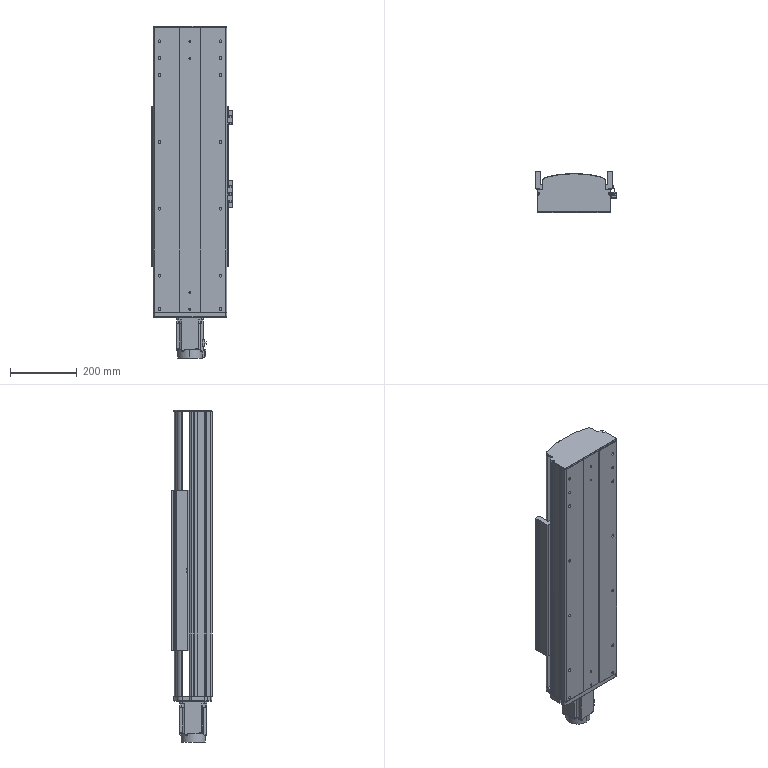Part | SolidWorks | features AEMSimFeature 1 | 30 solids | 1317 faces | box 242 x 122 x 992.2 mm | volume 12646217 mm3 | plane 687 | cylinder 492 | cone 82 | torus 56 | commonest cylinder face diameters 0.5 x36 5.5 x36 2.5 x32 1 x30 3 x28 8.6 x28